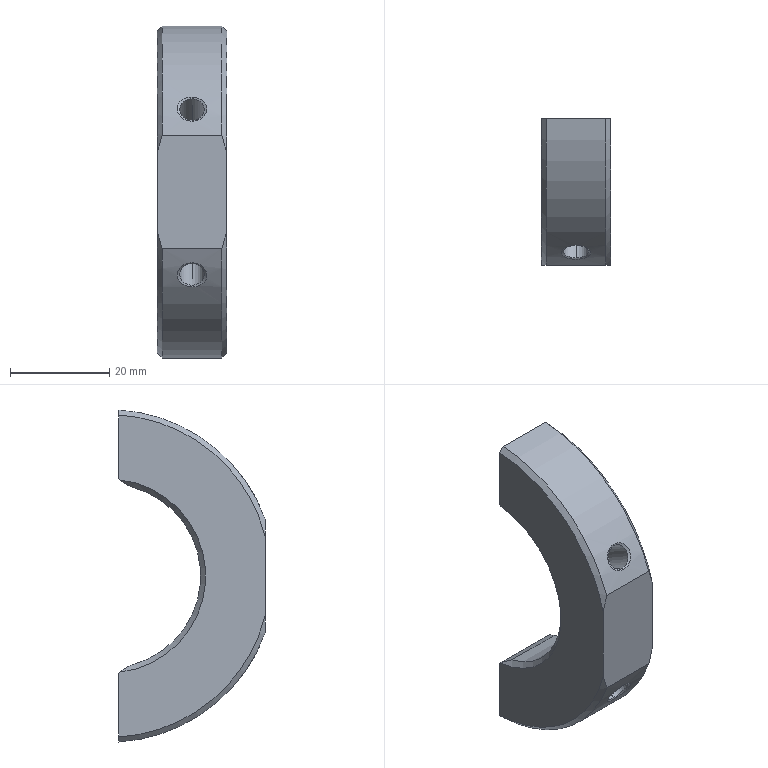Part | SolidWorks | features BaseBody 1 | 1 solid | 30 faces | box 14 x 29.5 x 66.88 mm | volume 15247 mm3 | cone 14 | plane 9 | cylinder 7 | commonest cylinder face diameters 5 x4 67 x2 37 x1
STEP:
#1=CARTESIAN_POINT('',(133.,-20.303,8.835));
#2=VERTEX_POINT('',#1);
#3=CARTESIAN_POINT('',(133.,-17.803,13.165));
#4=VERTEX_POINT('',#3);
#5=CARTESIAN_POINT('',(133.,-19.053,11.));
#6=DIRECTION('',(0.,-0.866,0.5));
#7=DIRECTION('',(0.,0.5,0.866));
#8=AXIS2_PLACEMENT_3D('',#5,#6,#7);
#9=CIRCLE('',#8,2.5);
#10=EDGE_CURVE('',#2,#4,#9,.T.);
#11=ORIENTED_EDGE('',*,*,#10,.F.);
#12=CARTESIAN_POINT('',(133.,-30.012,14.441));
#13=VERTEX_POINT('',#12);
#14=CARTESIAN_POINT('',(133.,-30.262,14.585));
#15=DIRECTION('',(0.,-0.866,0.5));
#16=VECTOR('',#15,1000.);
#17=LINE('',#14,#16);
#18=EDGE_CURVE('',#2,#13,#17,.T.);
#19=ORIENTED_EDGE('',*,*,#18,.T.);
#20=CARTESIAN_POINT('',(133.,-27.512,18.771));
#21=VERTEX_POINT('',#20);
#22=CARTESIAN_POINT('',(133.,-28.762,16.606));
#23=DIRECTION('',(0.,-0.866,0.5));
#24=DIRECTION('',(0.,0.5,0.866));
#25=AXIS2_PLACEMENT_3D('',#22,#23,#24);
#26=CIRCLE('',#25,2.5);
#27=EDGE_CURVE('',#13,#21,#26,.T.);
#28=ORIENTED_EDGE('',*,*,#27,.T.);
#29=CARTESIAN_POINT('',(133.,-27.762,18.915));
#30=DIRECTION('',(0.,-0.866,0.5));
#31=VECTOR('',#30,1000.);
#32=LINE('',#29,#31);
#33=EDGE_CURVE('',#4,#21,#32,.T.);
#34=ORIENTED_EDGE('',*,*,#33,.F.);
#35=EDGE_LOOP('',(#11,#19,#28,#34));
#36=FACE_OUTER_BOUND('',#35,.T.);
#37=CARTESIAN_POINT('',(133.,-29.012,16.75));
#38=DIRECTION('',(0.,-0.866,0.5));
#39=DIRECTION('',(0.,0.5,0.866));
#40=AXIS2_PLACEMENT_3D('',#37,#38,#39);
#41=CYLINDRICAL_SURFACE('',#40,2.5);
#42=ADVANCED_FACE('',(#36),#41,.F.);
#43=CARTESIAN_POINT('',(133.,-17.752,10.249));
#44=VERTEX_POINT('',#43);
#45=CARTESIAN_POINT('',(133.,-17.803,13.165));
#46=DIRECTION('',(0.,-0.01745,0.9998));
#47=VECTOR('',#46,1000.);
#48=LINE('',#45,#47);
#49=EDGE_CURVE('',#44,#4,#48,.T.);
#50=ORIENTED_EDGE('',*,*,#49,.F.);
#51=CARTESIAN_POINT('',(133.,-20.303,8.835));
#52=DIRECTION('',(0.,-0.8746,-0.4848));
#53=VECTOR('',#52,1000.);
#54=LINE('',#51,#53);
#55=EDGE_CURVE('',#44,#2,#54,.T.);
#56=ORIENTED_EDGE('',*,*,#55,.T.);
#57=ORIENTED_EDGE('',*,*,#10,.T.);
#58=EDGE_LOOP('',(#50,#56,#57));
#59=FACE_OUTER_BOUND('',#58,.T.);
#60=CARTESIAN_POINT('',(133.,-19.053,11.));
#61=DIRECTION('',(0.,-0.866,0.5));
#62=DIRECTION('',(0.,0.5,0.866));
#63=AXIS2_PLACEMENT_3D('',#60,#61,#62);
#64=CONICAL_SURFACE('',#63,2.5,1.03);
#65=ADVANCED_FACE('',(#59),#64,.F.);
#66=ORIENTED_EDGE('',*,*,#27,.F.);
#67=CARTESIAN_POINT('',(133.,-30.309,14.269));
#68=VERTEX_POINT('',#67);
#69=CARTESIAN_POINT('',(133.,-30.512,14.152));
#70=DIRECTION('',(0.,-0.866,-0.5));
#71=VECTOR('',#70,1000.);
#72=LINE('',#69,#71);
#73=EDGE_CURVE('',#13,#68,#72,.T.);
#74=ORIENTED_EDGE('',*,*,#73,.T.);
#75=CARTESIAN_POINT('',(133.,-27.512,19.114));
#76=VERTEX_POINT('',#75);
#77=CARTESIAN_POINT('',(133.,-27.512,19.114));
#78=CARTESIAN_POINT('',(133.19,-27.512,19.114));
#79=CARTESIAN_POINT('',(133.381,-27.522,19.1));
#80=CARTESIAN_POINT('',(133.753,-27.56,19.045));
#81=CARTESIAN_POINT('',(133.935,-27.588,19.004));
#82=CARTESIAN_POINT('',(134.292,-27.664,18.893));
#83=CARTESIAN_POINT('',(134.464,-27.711,18.824));
#84=CARTESIAN_POINT('',(134.787,-27.82,18.663));
#85=CARTESIAN_POINT('',(134.939,-27.883,18.57));
#86=CARTESIAN_POINT('',(135.224,-28.024,18.356));
#87=CARTESIAN_POINT('',(135.351,-28.1,18.238));
#88=CARTESIAN_POINT('',(135.576,-28.264,17.984));
#89=CARTESIAN_POINT('',(135.675,-28.352,17.845));
#90=CARTESIAN_POINT('',(135.835,-28.535,17.551));
#91=CARTESIAN_POINT('',(135.896,-28.628,17.399));
#92=CARTESIAN_POINT('',(135.978,-28.818,17.082));
#93=CARTESIAN_POINT('',(136.,-28.916,16.916));
#94=CARTESIAN_POINT('',(136.,-29.105,16.588));
#95=CARTESIAN_POINT('',(135.98,-29.198,16.425));
#96=CARTESIAN_POINT('',(135.897,-29.379,16.098));
#97=CARTESIAN_POINT('',(135.836,-29.465,15.939));
#98=CARTESIAN_POINT('',(135.599,-29.709,15.484));
#99=CARTESIAN_POINT('',(135.362,-29.853,15.203));
#100=CARTESIAN_POINT('',(134.94,-30.022,14.863));
#101=CARTESIAN_POINT('',(134.789,-30.072,14.763));
#102=CARTESIAN_POINT('',(134.463,-30.158,14.586));
#103=CARTESIAN_POINT('',(134.29,-30.194,14.511));
#104=CARTESIAN_POINT('',(133.76,-30.28,14.331));
#105=CARTESIAN_POINT('',(133.378,-30.309,14.269));
#106=CARTESIAN_POINT('',(133.,-30.309,14.269));
#107=B_SPLINE_CURVE_WITH_KNOTS('',3,(#77,#78,#79,#80,#81,#82,#83,#84,#85,#86,#87,#88,#89,#90,#91,#92,#93,#94,#95,#96,#97,#98,#99,#100,#101,#102,#103,#104,#105,#106),.UNSPECIFIED.,.F.,.F.,(4,2,2,2,2,2,2,2,2,2,2,2,2,2,4),(0.01163,0.01219,0.01276,0.01333,0.01389,0.01446,0.01503,0.01559,0.01616,0.01672,0.01729,0.01842,0.01899,0.01956,0.02069),.UNSPECIFIED.);
#108=EDGE_CURVE('',#76,#68,#107,.T.);
#109=ORIENTED_EDGE('',*,*,#108,.F.);
#110=CARTESIAN_POINT('',(133.,-27.512,19.348));
#111=DIRECTION('',(0.,0.,1.));
#112=VECTOR('',#111,1000.);
#113=LINE('',#110,#112);
#114=EDGE_CURVE('',#21,#76,#113,.T.);
#115=ORIENTED_EDGE('',*,*,#114,.F.);
#116=EDGE_LOOP('',(#66,#74,#109,#115));
#117=FACE_OUTER_BOUND('',#116,.T.);
#118=CARTESIAN_POINT('',(133.,-29.012,16.75));
#119=DIRECTION('',(0.,-0.866,0.5));
#120=DIRECTION('',(0.,0.5,0.866));
#121=AXIS2_PLACEMENT_3D('',#118,#119,#120);
#122=CONICAL_SURFACE('',#121,3.,1.047);
#123=ADVANCED_FACE('',(#117),#122,.F.);
#124=CARTESIAN_POINT('',(133.,-17.803,-13.165));
#125=VERTEX_POINT('',#124);
#126=CARTESIAN_POINT('',(133.,-20.303,-8.835));
#127=VERTEX_POINT('',#126);
#128=CARTESIAN_POINT('',(133.,-19.053,-11.));
#129=DIRECTION('',(0.,-0.866,-0.5));
#130=DIRECTION('',(0.,-0.5,0.866));
#131=AXIS2_PLACEMENT_3D('',#128,#129,#130);
#132=CIRCLE('',#131,2.5);
#133=EDGE_CURVE('',#125,#127,#132,.T.);
#134=ORIENTED_EDGE('',*,*,#133,.F.);
#135=CARTESIAN_POINT('',(133.,-27.512,-18.771));
#136=VERTEX_POINT('',#135);
#137=CARTESIAN_POINT('',(133.,-27.762,-18.915));
#138=DIRECTION('',(0.,-0.866,-0.5));
#139=VECTOR('',#138,1000.);
#140=LINE('',#137,#139);
#141=EDGE_CURVE('',#125,#136,#140,.T.);
#142=ORIENTED_EDGE('',*,*,#141,.T.);
#143=CARTESIAN_POINT('',(133.,-30.012,-14.441));
#144=VERTEX_POINT('',#143);
#145=CARTESIAN_POINT('',(133.,-28.762,-16.606));
#146=DIRECTION('',(0.,-0.866,-0.5));
#147=DIRECTION('',(0.,-0.5,0.866));
#148=AXIS2_PLACEMENT_3D('',#145,#146,#147);
#149=CIRCLE('',#148,2.5);
#150=EDGE_CURVE('',#136,#144,#149,.T.);
#151=ORIENTED_EDGE('',*,*,#150,.T.);
#152=CARTESIAN_POINT('',(133.,-30.262,-14.585));
#153=DIRECTION('',(0.,-0.866,-0.5));
#154=VECTOR('',#153,1000.);
#155=LINE('',#152,#154);
#156=EDGE_CURVE('',#127,#144,#155,.T.);
#157=ORIENTED_EDGE('',*,*,#156,.F.);
#158=EDGE_LOOP('',(#134,#142,#151,#157));
#159=FACE_OUTER_BOUND('',#158,.T.);
#160=CARTESIAN_POINT('',(133.,-29.012,-16.75));
#161=DIRECTION('',(0.,-0.866,-0.5));
#162=DIRECTION('',(0.,-0.5,0.866));
#163=AXIS2_PLACEMENT_3D('',#160,#161,#162);
#164=CYLINDRICAL_SURFACE('',#163,2.5);
#165=ADVANCED_FACE('',(#159),#164,.F.);
#166=CARTESIAN_POINT('',(133.,-17.752,-10.249));
#167=VERTEX_POINT('',#166);
#168=CARTESIAN_POINT('',(133.,-20.303,-8.835));
#169=DIRECTION('',(0.,-0.8746,0.4848));
#170=VECTOR('',#169,1000.);
#171=LINE('',#168,#170);
#172=EDGE_CURVE('',#167,#127,#171,.T.);
#173=ORIENTED_EDGE('',*,*,#172,.F.);
#174=CARTESIAN_POINT('',(133.,-17.803,-13.165));
#175=DIRECTION('',(0.,-0.01745,-0.9998));
#176=VECTOR('',#175,1000.);
#177=LINE('',#174,#176);
#178=EDGE_CURVE('',#167,#125,#177,.T.);
#179=ORIENTED_EDGE('',*,*,#178,.T.);
#180=ORIENTED_EDGE('',*,*,#133,.T.);
#181=EDGE_LOOP('',(#173,#179,#180));
#182=FACE_OUTER_BOUND('',#181,.T.);
#183=CARTESIAN_POINT('',(133.,-19.053,-11.));
#184=DIRECTION('',(0.,-0.866,-0.5));
#185=DIRECTION('',(0.,-0.5,0.866));
#186=AXIS2_PLACEMENT_3D('',#183,#184,#185);
#187=CONICAL_SURFACE('',#186,2.5,1.03);
#188=ADVANCED_FACE('',(#182),#187,.F.);
#189=ORIENTED_EDGE('',*,*,#150,.F.);
#190=CARTESIAN_POINT('',(133.,-27.512,-19.114));
#191=VERTEX_POINT('',#190);
#192=CARTESIAN_POINT('',(133.,-27.512,-19.348));
#193=DIRECTION('',(0.,0.,-1.));
#194=VECTOR('',#193,1000.);
#195=LINE('',#192,#194);
#196=EDGE_CURVE('',#136,#191,#195,.T.);
#197=ORIENTED_EDGE('',*,*,#196,.T.);
#198=CARTESIAN_POINT('',(133.,-30.309,-14.269));
#199=VERTEX_POINT('',#198);
#200=CARTESIAN_POINT('',(133.,-30.309,-14.269));
#201=CARTESIAN_POINT('',(133.19,-30.309,-14.269));
#202=CARTESIAN_POINT('',(133.378,-30.302,-14.284));
#203=CARTESIAN_POINT('',(133.75,-30.273,-14.345));
#204=CARTESIAN_POINT('',(133.936,-30.252,-14.391));
#205=CARTESIAN_POINT('',(134.292,-30.194,-14.511));
#206=CARTESIAN_POINT('',(134.461,-30.159,-14.585));
#207=CARTESIAN_POINT('',(134.785,-30.073,-14.761));
#208=CARTESIAN_POINT('',(134.941,-30.022,-14.864));
#209=CARTESIAN_POINT('',(135.222,-29.909,-15.09));
#210=CARTESIAN_POINT('',(135.349,-29.846,-15.214));
#211=CARTESIAN_POINT('',(135.576,-29.707,-15.485));
#212=CARTESIAN_POINT('',(135.675,-29.63,-15.631));
#213=CARTESIAN_POINT('',(135.834,-29.469,-15.934));
#214=CARTESIAN_POINT('',(135.895,-29.383,-16.091));
#215=CARTESIAN_POINT('',(135.979,-29.202,-16.417));
#216=CARTESIAN_POINT('',(136.,-29.108,-16.583));
#217=CARTESIAN_POINT('',(136.,-28.917,-16.914));
#218=CARTESIAN_POINT('',(135.979,-28.821,-17.078));
#219=CARTESIAN_POINT('',(135.897,-28.63,-17.395));
#220=CARTESIAN_POINT('',(135.835,-28.535,-17.551));
#221=CARTESIAN_POINT('',(135.676,-28.353,-17.843));
#222=CARTESIAN_POINT('',(135.579,-28.266,-17.981));
#223=CARTESIAN_POINT('',(135.352,-28.101,-18.238));
#224=CARTESIAN_POINT('',(135.222,-28.023,-18.356));
#225=CARTESIAN_POINT('',(134.942,-27.884,-18.568));
#226=CARTESIAN_POINT('',(134.787,-27.82,-18.663));
#227=CARTESIAN_POINT('',(134.461,-27.71,-18.826));
#228=CARTESIAN_POINT('',(134.291,-27.664,-18.893));
#229=CARTESIAN_POINT('',(133.936,-27.589,-19.003));
#230=CARTESIAN_POINT('',(133.751,-27.56,-19.045));
#231=CARTESIAN_POINT('',(133.378,-27.521,-19.1));
#232=CARTESIAN_POINT('',(133.19,-27.512,-19.114));
#233=CARTESIAN_POINT('',(133.,-27.512,-19.114));
#234=B_SPLINE_CURVE_WITH_KNOTS('',3,(#200,#201,#202,#203,#204,#205,#206,#207,#208,#209,#210,#211,#212,#213,#214,#215,#216,#217,#218,#219,#220,#221,#222,#223,#224,#225,#226,#227,#228,#229,#230,#231,#232,#233),.UNSPECIFIED.,.F.,.F.,(4,2,2,2,2,2,2,2,2,2,2,2,2,2,2,2,4),(0.01353,0.0141,0.01467,0.01523,0.0158,0.01637,0.01694,0.01751,0.01807,0.01864,0.01921,0.01978,0.02035,0.02091,0.02148,0.02205,0.02262),.UNSPECIFIED.);
#235=EDGE_CURVE('',#199,#191,#234,.T.);
#236=ORIENTED_EDGE('',*,*,#235,.F.);
#237=CARTESIAN_POINT('',(133.,-30.512,-14.152));
#238=DIRECTION('',(0.,-0.866,0.5));
#239=VECTOR('',#238,1000.);
#240=LINE('',#237,#239);
#241=EDGE_CURVE('',#144,#199,#240,.T.);
#242=ORIENTED_EDGE('',*,*,#241,.F.);
#243=EDGE_LOOP('',(#189,#197,#236,#242));
#244=FACE_OUTER_BOUND('',#243,.T.);
#245=CARTESIAN_POINT('',(133.,-29.012,-16.75));
#246=DIRECTION('',(0.,-0.866,-0.5));
#247=DIRECTION('',(0.,-0.5,0.866));
#248=AXIS2_PLACEMENT_3D('',#245,#246,#247);
#249=CONICAL_SURFACE('',#248,3.,1.047);
#250=ADVANCED_FACE('',(#244),#249,.F.);
#251=CARTESIAN_POINT('',(139.,-4.5,17.944));
#252=VERTEX_POINT('',#251);
#253=CARTESIAN_POINT('',(139.,-4.5,-17.944));
#254=VERTEX_POINT('',#253);
#255=CARTESIAN_POINT('',(139.,0.,0.));
#256=DIRECTION('',(1.,0.,0.));
#257=DIRECTION('',(0.,0.,1.));
#258=AXIS2_PLACEMENT_3D('',#255,#256,#257);
#259=CIRCLE('',#258,18.5);
#260=EDGE_CURVE('',#252,#254,#259,.T.);
#261=ORIENTED_EDGE('',*,*,#260,.T.);
#262=CARTESIAN_POINT('',(127.,-4.5,-17.944));
#263=VERTEX_POINT('',#262);
#264=CARTESIAN_POINT('',(140.,-4.5,-17.944));
#265=DIRECTION('',(-1.,0.,0.));
#266=VECTOR('',#265,1000.);
#267=LINE('',#264,#266);
#268=EDGE_CURVE('',#254,#263,#267,.T.);
#269=ORIENTED_EDGE('',*,*,#268,.T.);
#270=CARTESIAN_POINT('',(127.,-4.5,17.944));
#271=VERTEX_POINT('',#270);
#272=CARTESIAN_POINT('',(127.,0.,0.));
#273=DIRECTION('',(-1.,0.,0.));
#274=DIRECTION('',(0.,0.,1.));
#275=AXIS2_PLACEMENT_3D('',#272,#273,#274);
#276=CIRCLE('',#275,18.5);
#277=EDGE_CURVE('',#263,#271,#276,.T.);
#278=ORIENTED_EDGE('',*,*,#277,.T.);
#279=CARTESIAN_POINT('',(140.,-4.5,17.944));
#280=DIRECTION('',(-1.,0.,0.));
#281=VECTOR('',#280,1000.);
#282=LINE('',#279,#281);
#283=EDGE_CURVE('',#252,#271,#282,.T.);
#284=ORIENTED_EDGE('',*,*,#283,.F.);
#285=EDGE_LOOP('',(#261,#269,#278,#284));
#286=FACE_OUTER_BOUND('',#285,.T.);
#287=CARTESIAN_POINT('',(126.,0.,0.));
#288=DIRECTION('',(1.,0.,0.));
#289=DIRECTION('',(0.,0.,-1.));
#290=AXIS2_PLACEMENT_3D('',#287,#288,#289);
#291=CYLINDRICAL_SURFACE('',#290,18.5);
#292=ADVANCED_FACE('',(#286),#291,.F.);
#293=CARTESIAN_POINT('',(126.,-2.,-19.599));
#294=VERTEX_POINT('',#293);
#295=CARTESIAN_POINT('',(126.,-2.,-32.438));
#296=VERTEX_POINT('',#295);
#297=CARTESIAN_POINT('',(126.,-2.,-33.44));
#298=DIRECTION('',(0.,0.,-1.));
#299=VECTOR('',#298,1000.);
#300=LINE('',#297,#299);
#301=EDGE_CURVE('',#294,#296,#300,.T.);
#302=ORIENTED_EDGE('',*,*,#301,.F.);
#303=CARTESIAN_POINT('',(140.,-2.,-19.599));
#304=VERTEX_POINT('',#303);
#305=CARTESIAN_POINT('',(140.,-2.,-19.599));
#306=DIRECTION('',(-1.,0.,0.));
#307=VECTOR('',#306,1000.);
#308=LINE('',#305,#307);
#309=EDGE_CURVE('',#304,#294,#308,.T.);
#310=ORIENTED_EDGE('',*,*,#309,.F.);
#311=CARTESIAN_POINT('',(140.,-2.,-32.438));
#312=VERTEX_POINT('',#311);
#313=CARTESIAN_POINT('',(140.,-2.,-33.44));
#314=DIRECTION('',(0.,0.,-1.));
#315=VECTOR('',#314,1000.);
#316=LINE('',#313,#315);
#317=EDGE_CURVE('',#304,#312,#316,.T.);
#318=ORIENTED_EDGE('',*,*,#317,.T.);
#319=CARTESIAN_POINT('',(139.,-2.,-33.44));
#320=VERTEX_POINT('',#319);
#321=CARTESIAN_POINT('',(140.,-2.,-32.438));
#322=CARTESIAN_POINT('',(139.667,-2.,-32.772));
#323=CARTESIAN_POINT('',(139.333,-2.,-33.106));
#324=CARTESIAN_POINT('',(139.,-2.,-33.44));
#325=B_SPLINE_CURVE_WITH_KNOTS('',3,(#321,#322,#323,#324),.UNSPECIFIED.,.F.,.F.,(4,4),(0.,0.001416),.UNSPECIFIED.);
#326=EDGE_CURVE('',#312,#320,#325,.T.);
#327=ORIENTED_EDGE('',*,*,#326,.T.);
#328=CARTESIAN_POINT('',(127.,-2.,-33.44));
#329=VERTEX_POINT('',#328);
#330=CARTESIAN_POINT('',(126.,-2.,-33.44));
#331=DIRECTION('',(1.,0.,0.));
#332=VECTOR('',#331,1000.);
#333=LINE('',#330,#332);
#334=EDGE_CURVE('',#329,#320,#333,.T.);
#335=ORIENTED_EDGE('',*,*,#334,.F.);
#336=CARTESIAN_POINT('',(127.,-2.,-33.44));
#337=CARTESIAN_POINT('',(126.667,-2.,-33.106));
#338=CARTESIAN_POINT('',(126.333,-2.,-32.772));
#339=CARTESIAN_POINT('',(126.,-2.,-32.438));
#340=B_SPLINE_CURVE_WITH_KNOTS('',3,(#336,#337,#338,#339),.UNSPECIFIED.,.F.,.F.,(4,4),(0.,0.001416),.UNSPECIFIED.);
#341=EDGE_CURVE('',#329,#296,#340,.T.);
#342=ORIENTED_EDGE('',*,*,#341,.T.);
#343=EDGE_LOOP('',(#302,#310,#318,#327,#335,#342));
#344=FACE_OUTER_BOUND('',#343,.T.);
#345=CARTESIAN_POINT('',(126.,-2.,-33.44));
#346=DIRECTION('',(0.,-1.,0.));
#347=DIRECTION('',(1.,0.,0.));
#348=AXIS2_PLACEMENT_3D('',#345,#346,#347);
#349=PLANE('',#348);
#350=ADVANCED_FACE('',(#344),#349,.F.);
#351=ORIENTED_EDGE('',*,*,#235,.T.);
#352=CARTESIAN_POINT('',(133.,-27.512,-19.114));
#353=CARTESIAN_POINT('',(132.81,-27.512,-19.114));
#354=CARTESIAN_POINT('',(132.619,-27.522,-19.1));
#355=CARTESIAN_POINT('',(132.247,-27.56,-19.045));
#356=CARTESIAN_POINT('',(132.065,-27.588,-19.004));
#357=CARTESIAN_POINT('',(131.709,-27.664,-18.893));
#358=CARTESIAN_POINT('',(131.536,-27.711,-18.824));
#359=CARTESIAN_POINT('',(131.213,-27.82,-18.663));
#360=CARTESIAN_POINT('',(131.061,-27.883,-18.57));
#361=CARTESIAN_POINT('',(130.636,-28.094,-18.25));
#362=CARTESIAN_POINT('',(130.406,-28.26,-17.993));
#363=CARTESIAN_POINT('',(130.165,-28.535,-17.552));
#364=CARTESIAN_POINT('',(130.104,-28.628,-17.399));
#365=CARTESIAN_POINT('',(130.022,-28.818,-17.083));
#366=CARTESIAN_POINT('',(130.,-28.915,-16.917));
#367=CARTESIAN_POINT('',(130.,-29.105,-16.589));
#368=CARTESIAN_POINT('',(130.02,-29.198,-16.425));
#369=CARTESIAN_POINT('',(130.102,-29.379,-16.099));
#370=CARTESIAN_POINT('',(130.164,-29.465,-15.94));
#371=CARTESIAN_POINT('',(130.322,-29.627,-15.637));
#372=CARTESIAN_POINT('',(130.42,-29.704,-15.49));
#373=CARTESIAN_POINT('',(130.647,-29.844,-15.218));
#374=CARTESIAN_POINT('',(130.774,-29.907,-15.094));
#375=CARTESIAN_POINT('',(131.056,-30.021,-14.865));
#376=CARTESIAN_POINT('',(131.211,-30.072,-14.763));
#377=CARTESIAN_POINT('',(131.535,-30.158,-14.587));
#378=CARTESIAN_POINT('',(131.706,-30.194,-14.512));
#379=CARTESIAN_POINT('',(132.064,-30.252,-14.391));
#380=CARTESIAN_POINT('',(132.247,-30.273,-14.345));
#381=CARTESIAN_POINT('',(132.619,-30.302,-14.285));
#382=CARTESIAN_POINT('',(132.81,-30.309,-14.269));
#383=CARTESIAN_POINT('',(133.,-30.309,-14.269));
#384=B_SPLINE_CURVE_WITH_KNOTS('',3,(#352,#353,#354,#355,#356,#357,#358,#359,#360,#361,#362,#363,#364,#365,#366,#367,#368,#369,#370,#371,#372,#373,#374,#375,#376,#377,#378,#379,#380,#381,#382,#383),.UNSPECIFIED.,.F.,.F.,(4,2,2,2,2,2,2,2,2,2,2,2,2,2,2,4),(0.004439,0.005007,0.005576,0.006144,0.006712,0.007848,0.008416,0.008984,0.009552,0.01012,0.01069,0.01126,0.01182,0.01239,0.01296,0.01353),.UNSPECIFIED.);
#385=EDGE_CURVE('',#191,#199,#384,.T.);
#386=ORIENTED_EDGE('',*,*,#385,.T.);
#387=EDGE_LOOP('',(#351,#386));
#388=FACE_BOUND('',#387,.T.);
#389=ORIENTED_EDGE('',*,*,#334,.T.);
#390=CARTESIAN_POINT('',(139.,-31.5,-11.402));
#391=VERTEX_POINT('',#390);
#392=CARTESIAN_POINT('',(139.,0.,0.));
#393=DIRECTION('',(-1.,0.,0.));
#394=DIRECTION('',(0.,0.,1.));
#395=AXIS2_PLACEMENT_3D('',#392,#393,#394);
#396=CIRCLE('',#395,33.5);
#397=EDGE_CURVE('',#320,#391,#396,.T.);
#398=ORIENTED_EDGE('',*,*,#397,.T.);
#399=CARTESIAN_POINT('',(127.,-31.5,-11.402));
#400=VERTEX_POINT('',#399);
#401=CARTESIAN_POINT('',(126.,-31.5,-11.402));
#402=DIRECTION('',(1.,0.,0.));
#403=VECTOR('',#402,1000.);
#404=LINE('',#401,#403);
#405=EDGE_CURVE('',#400,#391,#404,.T.);
#406=ORIENTED_EDGE('',*,*,#405,.F.);
#407=CARTESIAN_POINT('',(127.,0.,0.));
#408=DIRECTION('',(1.,0.,0.));
#409=DIRECTION('',(0.,0.,1.));
#410=AXIS2_PLACEMENT_3D('',#407,#408,#409);
#411=CIRCLE('',#410,33.5);
#412=EDGE_CURVE('',#400,#329,#411,.T.);
#413=ORIENTED_EDGE('',*,*,#412,.T.);
#414=EDGE_LOOP('',(#389,#398,#406,#413));
#415=FACE_OUTER_BOUND('',#414,.T.);
#416=CARTESIAN_POINT('',(126.,0.,0.));
#417=DIRECTION('',(1.,0.,0.));
#418=DIRECTION('',(0.,0.,-1.));
#419=AXIS2_PLACEMENT_3D('',#416,#417,#418);
#420=CYLINDRICAL_SURFACE('',#419,33.5);
#421=ADVANCED_FACE('',(#388,#415),#420,.T.);
#422=CARTESIAN_POINT('',(140.,-31.5,-8.));
#423=VERTEX_POINT('',#422);
#424=CARTESIAN_POINT('',(140.,-31.5,8.));
#425=VERTEX_POINT('',#424);
#426=CARTESIAN_POINT('',(140.,-31.5,-11.402));
#427=DIRECTION('',(0.,0.,1.));
#428=VECTOR('',#427,1000.);
#429=LINE('',#426,#428);
#430=EDGE_CURVE('',#423,#425,#429,.T.);
#431=ORIENTED_EDGE('',*,*,#430,.T.);
#432=CARTESIAN_POINT('',(139.,-31.5,11.402));
#433=VERTEX_POINT('',#432);
#434=CARTESIAN_POINT('',(140.,-31.5,8.));
#435=CARTESIAN_POINT('',(139.717,-31.5,9.149));
#436=CARTESIAN_POINT('',(139.381,-31.5,10.282));
#437=CARTESIAN_POINT('',(139.,-31.5,11.402));
#438=B_SPLINE_CURVE_WITH_KNOTS('',3,(#434,#435,#436,#437),.UNSPECIFIED.,.F.,.F.,(4,4),(0.,0.003546),.UNSPECIFIED.);
#439=EDGE_CURVE('',#425,#433,#438,.T.);
#440=ORIENTED_EDGE('',*,*,#439,.T.);
#441=CARTESIAN_POINT('',(127.,-31.5,11.402));
#442=VERTEX_POINT('',#441);
#443=CARTESIAN_POINT('',(126.,-31.5,11.402));
#444=DIRECTION('',(1.,0.,0.));
#445=VECTOR('',#444,1000.);
#446=LINE('',#443,#445);
#447=EDGE_CURVE('',#442,#433,#446,.T.);
#448=ORIENTED_EDGE('',*,*,#447,.F.);
#449=CARTESIAN_POINT('',(126.,-31.5,8.));
#450=VERTEX_POINT('',#449);
#451=CARTESIAN_POINT('',(127.,-31.5,11.402));
#452=CARTESIAN_POINT('',(126.619,-31.5,10.282));
#453=CARTESIAN_POINT('',(126.283,-31.5,9.149));
#454=CARTESIAN_POINT('',(126.,-31.5,8.));
#455=B_SPLINE_CURVE_WITH_KNOTS('',3,(#451,#452,#453,#454),.UNSPECIFIED.,.F.,.F.,(4,4),(0.,0.003546),.UNSPECIFIED.);
#456=EDGE_CURVE('',#442,#450,#455,.T.);
#457=ORIENTED_EDGE('',*,*,#456,.T.);
#458=CARTESIAN_POINT('',(126.,-31.5,-8.));
#459=VERTEX_POINT('',#458);
#460=CARTESIAN_POINT('',(126.,-31.5,-11.402));
#461=DIRECTION('',(0.,0.,1.));
#462=VECTOR('',#461,1000.);
#463=LINE('',#460,#462);
#464=EDGE_CURVE('',#459,#450,#463,.T.);
#465=ORIENTED_EDGE('',*,*,#464,.F.);
#466=CARTESIAN_POINT('',(126.,-31.5,-8.));
#467=CARTESIAN_POINT('',(126.283,-31.5,-9.149));
#468=CARTESIAN_POINT('',(126.619,-31.5,-10.282));
#469=CARTESIAN_POINT('',(127.,-31.5,-11.402));
#470=B_SPLINE_CURVE_WITH_KNOTS('',3,(#466,#467,#468,#469),.UNSPECIFIED.,.F.,.F.,(4,4),(0.,0.003546),.UNSPECIFIED.);
#471=EDGE_CURVE('',#459,#400,#470,.T.);
#472=ORIENTED_EDGE('',*,*,#471,.T.);
#473=ORIENTED_EDGE('',*,*,#405,.T.);
#474=CARTESIAN_POINT('',(139.,-31.5,-11.402));
#475=CARTESIAN_POINT('',(139.381,-31.5,-10.282));
#476=CARTESIAN_POINT('',(139.717,-31.5,-9.149));
#477=CARTESIAN_POINT('',(140.,-31.5,-8.));
#478=B_SPLINE_CURVE_WITH_KNOTS('',3,(#474,#475,#476,#477),.UNSPECIFIED.,.F.,.F.,(4,4),(0.,0.003546),.UNSPECIFIED.);
#479=EDGE_CURVE('',#391,#423,#478,.T.);
#480=ORIENTED_EDGE('',*,*,#479,.T.);
#481=EDGE_LOOP('',(#431,#440,#448,#457,#465,#472,#473,#480));
#482=FACE_OUTER_BOUND('',#481,.T.);
#483=CARTESIAN_POINT('',(126.,-31.5,-11.402));
#484=DIRECTION('',(0.,1.,0.));
#485=DIRECTION('',(-1.,0.,0.));
#486=AXIS2_PLACEMENT_3D('',#483,#484,#485);
#487=PLANE('',#486);
#488=ADVANCED_FACE('',(#482),#487,.F.);
#489=ORIENTED_EDGE('',*,*,#108,.T.);
#490=CARTESIAN_POINT('',(133.,-30.309,14.269));
#491=CARTESIAN_POINT('',(132.811,-30.309,14.269));
#492=CARTESIAN_POINT('',(132.621,-30.302,14.284));
#493=CARTESIAN_POINT('',(132.246,-30.273,14.346));
#494=CARTESIAN_POINT('',(132.063,-30.252,14.391));
#495=CARTESIAN_POINT('',(131.71,-30.194,14.511));
#496=CARTESIAN_POINT('',(131.537,-30.158,14.586));
#497=CARTESIAN_POINT('',(131.211,-30.072,14.762));
#498=CARTESIAN_POINT('',(131.06,-30.023,14.863));
#499=CARTESIAN_POINT('',(130.779,-29.91,15.089));
#500=CARTESIAN_POINT('',(130.649,-29.845,15.216));
#501=CARTESIAN_POINT('',(130.423,-29.706,15.487));
#502=CARTESIAN_POINT('',(130.326,-29.631,15.63));
#503=CARTESIAN_POINT('',(130.166,-29.469,15.934));
#504=CARTESIAN_POINT('',(130.104,-29.381,16.094));
#505=CARTESIAN_POINT('',(130.022,-29.202,16.417));
#506=CARTESIAN_POINT('',(130.,-29.11,16.581));
#507=CARTESIAN_POINT('',(130.,-28.918,16.913));
#508=CARTESIAN_POINT('',(130.02,-28.822,17.075));
#509=CARTESIAN_POINT('',(130.102,-28.632,17.392));
#510=CARTESIAN_POINT('',(130.164,-28.536,17.549));
#511=CARTESIAN_POINT('',(130.402,-28.263,17.987));
#512=CARTESIAN_POINT('',(130.635,-28.094,18.249));
#513=CARTESIAN_POINT('',(131.057,-27.884,18.567));
#514=CARTESIAN_POINT('',(131.212,-27.821,18.662));
#515=CARTESIAN_POINT('',(131.537,-27.711,18.825));
#516=CARTESIAN_POINT('',(131.708,-27.664,18.893));
#517=CARTESIAN_POINT('',(132.063,-27.589,19.003));
#518=CARTESIAN_POINT('',(132.249,-27.56,19.045));
#519=CARTESIAN_POINT('',(132.621,-27.521,19.1));
#520=CARTESIAN_POINT('',(132.81,-27.512,19.114));
#521=CARTESIAN_POINT('',(133.,-27.512,19.114));
#522=B_SPLINE_CURVE_WITH_KNOTS('',3,(#490,#491,#492,#493,#494,#495,#496,#497,#498,#499,#500,#501,#502,#503,#504,#505,#506,#507,#508,#509,#510,#511,#512,#513,#514,#515,#516,#517,#518,#519,#520,#521),.UNSPECIFIED.,.F.,.F.,(4,2,2,2,2,2,2,2,2,2,2,2,2,2,2,4),(0.002561,0.003128,0.003694,0.004261,0.004828,0.005394,0.005961,0.006527,0.007094,0.007661,0.008227,0.009361,0.009927,0.01049,0.01106,0.01163),.UNSPECIFIED.);
#523=EDGE_CURVE('',#68,#76,#522,.T.);
#524=ORIENTED_EDGE('',*,*,#523,.T.);
#525=EDGE_LOOP('',(#489,#524));
#526=FACE_BOUND('',#525,.T.);
#527=ORIENTED_EDGE('',*,*,#447,.T.);
#528=CARTESIAN_POINT('',(139.,-2.,33.44));
#529=VERTEX_POINT('',#528);
#530=CARTESIAN_POINT('',(139.,0.,0.));
#531=DIRECTION('',(-1.,0.,0.));
#532=DIRECTION('',(0.,0.,1.));
#533=AXIS2_PLACEMENT_3D('',#530,#531,#532);
#534=CIRCLE('',#533,33.5);
#535=EDGE_CURVE('',#433,#529,#534,.T.);
#536=ORIENTED_EDGE('',*,*,#535,.T.);
#537=CARTESIAN_POINT('',(127.,-2.,33.44));
#538=VERTEX_POINT('',#537);
#539=CARTESIAN_POINT('',(126.,-2.,33.44));
#540=DIRECTION('',(1.,0.,0.));
#541=VECTOR('',#540,1000.);
#542=LINE('',#539,#541);
#543=EDGE_CURVE('',#538,#529,#542,.T.);
#544=ORIENTED_EDGE('',*,*,#543,.F.);
#545=CARTESIAN_POINT('',(127.,0.,0.));
#546=DIRECTION('',(1.,0.,0.));
#547=DIRECTION('',(0.,0.,1.));
#548=AXIS2_PLACEMENT_3D('',#545,#546,#547);
#549=CIRCLE('',#548,33.5);
#550=EDGE_CURVE('',#538,#442,#549,.T.);
#551=ORIENTED_EDGE('',*,*,#550,.T.);
#552=EDGE_LOOP('',(#527,#536,#544,#551));
#553=FACE_OUTER_BOUND('',#552,.T.);
#554=CARTESIAN_POINT('',(126.,0.,0.));
#555=DIRECTION('',(1.,0.,0.));
#556=DIRECTION('',(0.,0.,-1.));
#557=AXIS2_PLACEMENT_3D('',#554,#555,#556);
#558=CYLINDRICAL_SURFACE('',#557,33.5);
#559=ADVANCED_FACE('',(#526,#553),#558,.T.);
#560=CARTESIAN_POINT('',(140.,-2.,32.438));
#561=VERTEX_POINT('',#560);
#562=CARTESIAN_POINT('',(140.,-2.,19.599));
#563=VERTEX_POINT('',#562);
#564=CARTESIAN_POINT('',(140.,-2.,18.392));
#565=DIRECTION('',(0.,0.,-1.));
#566=VECTOR('',#565,1000.);
#567=LINE('',#564,#566);
#568=EDGE_CURVE('',#561,#563,#567,.T.);
#569=ORIENTED_EDGE('',*,*,#568,.T.);
#570=CARTESIAN_POINT('',(126.,-2.,19.599));
#571=VERTEX_POINT('',#570);
#572=CARTESIAN_POINT('',(140.,-2.,19.599));
#573=DIRECTION('',(-1.,0.,0.));
#574=VECTOR('',#573,1000.);
#575=LINE('',#572,#574);
#576=EDGE_CURVE('',#563,#571,#575,.T.);
#577=ORIENTED_EDGE('',*,*,#576,.T.);
#578=CARTESIAN_POINT('',(126.,-2.,32.438));
#579=VERTEX_POINT('',#578);
#580=CARTESIAN_POINT('',(126.,-2.,18.392));
#581=DIRECTION('',(0.,0.,-1.));
#582=VECTOR('',#581,1000.);
#583=LINE('',#580,#582);
#584=EDGE_CURVE('',#579,#571,#583,.T.);
#585=ORIENTED_EDGE('',*,*,#584,.F.);
#586=CARTESIAN_POINT('',(126.,-2.,32.438));
#587=CARTESIAN_POINT('',(126.333,-2.,32.772));
#588=CARTESIAN_POINT('',(126.667,-2.,33.106));
#589=CARTESIAN_POINT('',(127.,-2.,33.44));
#590=B_SPLINE_CURVE_WITH_KNOTS('',3,(#586,#587,#588,#589),.UNSPECIFIED.,.F.,.F.,(4,4),(0.,0.001416),.UNSPECIFIED.);
#591=EDGE_CURVE('',#579,#538,#590,.T.);
#592=ORIENTED_EDGE('',*,*,#591,.T.);
#593=ORIENTED_EDGE('',*,*,#543,.T.);
#594=CARTESIAN_POINT('',(139.,-2.,33.44));
#595=CARTESIAN_POINT('',(139.333,-2.,33.106));
#596=CARTESIAN_POINT('',(139.667,-2.,32.772));
#597=CARTESIAN_POINT('',(140.,-2.,32.438));
#598=B_SPLINE_CURVE_WITH_KNOTS('',3,(#594,#595,#596,#597),.UNSPECIFIED.,.F.,.F.,(4,4),(0.,0.001416),.UNSPECIFIED.);
#599=EDGE_CURVE('',#529,#561,#598,.T.);
#600=ORIENTED_EDGE('',*,*,#599,.T.);
#601=EDGE_LOOP('',(#569,#577,#585,#592,#593,#600));
#602=FACE_OUTER_BOUND('',#601,.T.);
#603=CARTESIAN_POINT('',(126.,-2.,18.392));
#604=DIRECTION('',(0.,-1.,0.));
#605=DIRECTION('',(1.,0.,0.));
#606=AXIS2_PLACEMENT_3D('',#603,#604,#605);
#607=PLANE('',#606);
#608=ADVANCED_FACE('',(#602),#607,.F.);
#609=CARTESIAN_POINT('',(126.,-2.227,-19.372));
#610=VERTEX_POINT('',#609);
#611=CARTESIAN_POINT('',(126.,-2.5,-19.099));
#612=DIRECTION('',(0.,-0.7071,0.7071));
#613=VECTOR('',#612,1000.);
#614=LINE('',#611,#613);
#615=EDGE_CURVE('',#294,#610,#614,.T.);
#616=ORIENTED_EDGE('',*,*,#615,.F.);
#617=ORIENTED_EDGE('',*,*,#301,.T.);
#618=CARTESIAN_POINT('',(126.,0.,0.));
#619=DIRECTION('',(-1.,0.,0.));
#620=DIRECTION('',(0.,0.,1.));
#621=AXIS2_PLACEMENT_3D('',#618,#619,#620);
#622=CIRCLE('',#621,32.5);
#623=EDGE_CURVE('',#296,#459,#622,.T.);
#624=ORIENTED_EDGE('',*,*,#623,.T.);
#625=ORIENTED_EDGE('',*,*,#464,.T.);
#626=CARTESIAN_POINT('',(126.,0.,0.));
#627=DIRECTION('',(-1.,0.,0.));
#628=DIRECTION('',(0.,0.,1.));
#629=AXIS2_PLACEMENT_3D('',#626,#627,#628);
#630=CIRCLE('',#629,32.5);
#631=EDGE_CURVE('',#450,#579,#630,.T.);
#632=ORIENTED_EDGE('',*,*,#631,.T.);
#633=ORIENTED_EDGE('',*,*,#584,.T.);
#634=CARTESIAN_POINT('',(126.,-2.227,19.372));
#635=VERTEX_POINT('',#634);
#636=CARTESIAN_POINT('',(126.,-2.5,19.099));
#637=DIRECTION('',(0.,0.7071,0.7071));
#638=VECTOR('',#637,1000.);
#639=LINE('',#636,#638);
#640=EDGE_CURVE('',#635,#571,#639,.T.);
#641=ORIENTED_EDGE('',*,*,#640,.F.);
#642=CARTESIAN_POINT('',(126.,0.,0.));
#643=DIRECTION('',(1.,0.,0.));
#644=DIRECTION('',(0.,0.,1.));
#645=AXIS2_PLACEMENT_3D('',#642,#643,#644);
#646=CIRCLE('',#645,19.5);
#647=EDGE_CURVE('',#635,#610,#646,.T.);
#648=ORIENTED_EDGE('',*,*,#647,.T.);
#649=EDGE_LOOP('',(#616,#617,#624,#625,#632,#633,#641,#648));
#650=FACE_OUTER_BOUND('',#649,.T.);
#651=CARTESIAN_POINT('',(126.,0.,0.));
#652=DIRECTION('',(-1.,0.,0.));
#653=DIRECTION('',(0.,0.,1.));
#654=AXIS2_PLACEMENT_3D('',#651,#652,#653);
#655=PLANE('',#654);
#656=ADVANCED_FACE('',(#650),#655,.T.);
#657=ORIENTED_EDGE('',*,*,#317,.F.);
#658=CARTESIAN_POINT('',(140.,-2.227,-19.372));
#659=VERTEX_POINT('',#658);
#660=CARTESIAN_POINT('',(140.,-2.5,-19.099));
#661=DIRECTION('',(0.,-0.7071,0.7071));
#662=VECTOR('',#661,1000.);
#663=LINE('',#660,#662);
#664=EDGE_CURVE('',#304,#659,#663,.T.);
#665=ORIENTED_EDGE('',*,*,#664,.T.);
#666=CARTESIAN_POINT('',(140.,-2.227,19.372));
#667=VERTEX_POINT('',#666);
#668=CARTESIAN_POINT('',(140.,0.,0.));
#669=DIRECTION('',(-1.,0.,0.));
#670=DIRECTION('',(0.,0.,1.));
#671=AXIS2_PLACEMENT_3D('',#668,#669,#670);
#672=CIRCLE('',#671,19.5);
#673=EDGE_CURVE('',#659,#667,#672,.T.);
#674=ORIENTED_EDGE('',*,*,#673,.T.);
#675=CARTESIAN_POINT('',(140.,-2.5,19.099));
#676=DIRECTION('',(0.,0.7071,0.7071));
#677=VECTOR('',#676,1000.);
#678=LINE('',#675,#677);
#679=EDGE_CURVE('',#667,#563,#678,.T.);
#680=ORIENTED_EDGE('',*,*,#679,.T.);
#681=ORIENTED_EDGE('',*,*,#568,.F.);
#682=CARTESIAN_POINT('',(140.,0.,0.));
#683=DIRECTION('',(1.,0.,0.));
#684=DIRECTION('',(0.,0.,1.));
#685=AXIS2_PLACEMENT_3D('',#682,#683,#684);
#686=CIRCLE('',#685,32.5);
#687=EDGE_CURVE('',#561,#425,#686,.T.);
#688=ORIENTED_EDGE('',*,*,#687,.T.);
#689=ORIENTED_EDGE('',*,*,#430,.F.);
#690=CARTESIAN_POINT('',(140.,0.,0.));
#691=DIRECTION('',(1.,0.,0.));
#692=DIRECTION('',(0.,0.,1.));
#693=AXIS2_PLACEMENT_3D('',#690,#691,#692);
#694=CIRCLE('',#693,32.5);
#695=EDGE_CURVE('',#423,#312,#694,.T.);
#696=ORIENTED_EDGE('',*,*,#695,.T.);
#697=EDGE_LOOP('',(#657,#665,#674,#680,#681,#688,#689,#696));
#698=FACE_OUTER_BOUND('',#697,.T.);
#699=CARTESIAN_POINT('',(140.,0.,0.));
#700=DIRECTION('',(-1.,0.,0.));
#701=DIRECTION('',(0.,0.,1.));
#702=AXIS2_PLACEMENT_3D('',#699,#700,#701);
#703=PLANE('',#702);
#704=ADVANCED_FACE('',(#698),#703,.F.);
#705=CARTESIAN_POINT('',(126.238,-2.5,-19.099));
#706=VERTEX_POINT('',#705);
#707=CARTESIAN_POINT('',(126.238,-2.5,-19.099));
#708=CARTESIAN_POINT('',(126.529,-3.156,-18.72));
#709=CARTESIAN_POINT('',(126.785,-3.822,-18.336));
#710=CARTESIAN_POINT('',(127.,-4.5,-17.944));
#711=B_SPLINE_CURVE_WITH_KNOTS('',3,(#707,#708,#709,#710),.UNSPECIFIED.,.F.,.F.,(4,4),(0.000000247,0.002432),.UNSPECIFIED.);
#712=EDGE_CURVE('',#706,#263,#711,.T.);
#713=ORIENTED_EDGE('',*,*,#712,.F.);
#714=CARTESIAN_POINT('',(126.,-2.227,-19.372));
#715=CARTESIAN_POINT('',(126.08,-2.317,-19.282));
#716=CARTESIAN_POINT('',(126.159,-2.409,-19.19));
#717=CARTESIAN_POINT('',(126.238,-2.5,-19.099));
#718=B_SPLINE_CURVE_WITH_KNOTS('',3,(#714,#715,#716,#717),.UNSPECIFIED.,.F.,.F.,(4,4),(0.000000379,0.0004544),.UNSPECIFIED.);
#719=EDGE_CURVE('',#610,#706,#718,.T.);
#720=ORIENTED_EDGE('',*,*,#719,.F.);
#721=ORIENTED_EDGE('',*,*,#647,.F.);
#722=CARTESIAN_POINT('',(126.238,-2.5,19.099));
#723=VERTEX_POINT('',#722);
#724=CARTESIAN_POINT('',(126.238,-2.5,19.099));
#725=CARTESIAN_POINT('',(126.159,-2.409,19.19));
#726=CARTESIAN_POINT('',(126.08,-2.317,19.282));
#727=CARTESIAN_POINT('',(126.,-2.227,19.372));
#728=B_SPLINE_CURVE_WITH_KNOTS('',3,(#724,#725,#726,#727),.UNSPECIFIED.,.F.,.F.,(4,4),(0.000000331,0.0004544),.UNSPECIFIED.);
#729=EDGE_CURVE('',#723,#635,#728,.T.);
#730=ORIENTED_EDGE('',*,*,#729,.F.);
#731=CARTESIAN_POINT('',(127.,-4.5,17.944));
#732=CARTESIAN_POINT('',(126.785,-3.822,18.336));
#733=CARTESIAN_POINT('',(126.529,-3.156,18.72));
#734=CARTESIAN_POINT('',(126.238,-2.5,19.099));
#735=B_SPLINE_CURVE_WITH_KNOTS('',3,(#731,#732,#733,#734),.UNSPECIFIED.,.F.,.F.,(4,4),(0.000000239,0.002432),.UNSPECIFIED.);
#736=EDGE_CURVE('',#271,#723,#735,.T.);
#737=ORIENTED_EDGE('',*,*,#736,.F.);
#738=ORIENTED_EDGE('',*,*,#277,.F.);
#739=EDGE_LOOP('',(#713,#720,#721,#730,#737,#738));
#740=FACE_OUTER_BOUND('',#739,.T.);
#741=CARTESIAN_POINT('',(126.,0.,0.));
#742=DIRECTION('',(-1.,0.,0.));
#743=DIRECTION('',(0.,0.,1.));
#744=AXIS2_PLACEMENT_3D('',#741,#742,#743);
#745=CONICAL_SURFACE('',#744,19.5,0.7854);
#746=ADVANCED_FACE('',(#740),#745,.F.);
#747=CARTESIAN_POINT('',(139.762,-2.5,-19.099));
#748=VERTEX_POINT('',#747);
#749=CARTESIAN_POINT('',(139.,-4.5,-17.944));
#750=CARTESIAN_POINT('',(139.215,-3.822,-18.336));
#751=CARTESIAN_POINT('',(139.471,-3.156,-18.72));
#752=CARTESIAN_POINT('',(139.762,-2.5,-19.099));
#753=B_SPLINE_CURVE_WITH_KNOTS('',3,(#749,#750,#751,#752),.UNSPECIFIED.,.F.,.F.,(4,4),(0.000000239,0.002432),.UNSPECIFIED.);
#754=EDGE_CURVE('',#254,#748,#753,.T.);
#755=ORIENTED_EDGE('',*,*,#754,.F.);
#756=ORIENTED_EDGE('',*,*,#260,.F.);
#757=CARTESIAN_POINT('',(139.762,-2.5,19.099));
#758=VERTEX_POINT('',#757);
#759=CARTESIAN_POINT('',(139.762,-2.5,19.099));
#760=CARTESIAN_POINT('',(139.471,-3.156,18.72));
#761=CARTESIAN_POINT('',(139.215,-3.822,18.336));
#762=CARTESIAN_POINT('',(139.,-4.5,17.944));
#763=B_SPLINE_CURVE_WITH_KNOTS('',3,(#759,#760,#761,#762),.UNSPECIFIED.,.F.,.F.,(4,4),(0.000000247,0.002432),.UNSPECIFIED.);
#764=EDGE_CURVE('',#758,#252,#763,.T.);
#765=ORIENTED_EDGE('',*,*,#764,.F.);
#766=CARTESIAN_POINT('',(140.,-2.227,19.372));
#767=CARTESIAN_POINT('',(139.92,-2.317,19.282));
#768=CARTESIAN_POINT('',(139.841,-2.409,19.19));
#769=CARTESIAN_POINT('',(139.762,-2.5,19.099));
#770=B_SPLINE_CURVE_WITH_KNOTS('',3,(#766,#767,#768,#769),.UNSPECIFIED.,.F.,.F.,(4,4),(0.000000379,0.0004544),.UNSPECIFIED.);
#771=EDGE_CURVE('',#667,#758,#770,.T.);
#772=ORIENTED_EDGE('',*,*,#771,.F.);
#773=ORIENTED_EDGE('',*,*,#673,.F.);
#774=CARTESIAN_POINT('',(139.762,-2.5,-19.099));
#775=CARTESIAN_POINT('',(139.841,-2.409,-19.19));
#776=CARTESIAN_POINT('',(139.92,-2.317,-19.282));
#777=CARTESIAN_POINT('',(140.,-2.227,-19.372));
#778=B_SPLINE_CURVE_WITH_KNOTS('',3,(#774,#775,#776,#777),.UNSPECIFIED.,.F.,.F.,(4,4),(0.000000331,0.0004544),.UNSPECIFIED.);
#779=EDGE_CURVE('',#748,#659,#778,.T.);
#780=ORIENTED_EDGE('',*,*,#779,.F.);
#781=EDGE_LOOP('',(#755,#756,#765,#772,#773,#780));
#782=FACE_OUTER_BOUND('',#781,.T.);
#783=CARTESIAN_POINT('',(139.,0.,0.));
#784=DIRECTION('',(1.,0.,0.));
#785=DIRECTION('',(0.,0.,-1.));
#786=AXIS2_PLACEMENT_3D('',#783,#784,#785);
#787=CONICAL_SURFACE('',#786,18.5,0.7854);
#788=ADVANCED_FACE('',(#782),#787,.F.);
#789=ORIENTED_EDGE('',*,*,#439,.F.);
#790=ORIENTED_EDGE('',*,*,#687,.F.);
#791=ORIENTED_EDGE('',*,*,#599,.F.);
#792=ORIENTED_EDGE('',*,*,#535,.F.);
#793=EDGE_LOOP('',(#789,#790,#791,#792));
#794=FACE_OUTER_BOUND('',#793,.T.);
#795=CARTESIAN_POINT('',(139.,0.,0.));
#796=DIRECTION('',(-1.,0.,0.));
#797=DIRECTION('',(0.,0.,1.));
#798=AXIS2_PLACEMENT_3D('',#795,#796,#797);
#799=CONICAL_SURFACE('',#798,33.5,0.7854);
#800=ADVANCED_FACE('',(#794),#799,.T.);
#801=ORIENTED_EDGE('',*,*,#456,.F.);
#802=ORIENTED_EDGE('',*,*,#550,.F.);
#803=ORIENTED_EDGE('',*,*,#591,.F.);
#804=ORIENTED_EDGE('',*,*,#631,.F.);
#805=EDGE_LOOP('',(#801,#802,#803,#804));
#806=FACE_OUTER_BOUND('',#805,.T.);
#807=CARTESIAN_POINT('',(126.,0.,0.));
#808=DIRECTION('',(1.,0.,0.));
#809=DIRECTION('',(0.,0.,-1.));
#810=AXIS2_PLACEMENT_3D('',#807,#808,#809);
#811=CONICAL_SURFACE('',#810,32.5,0.7854);
#812=ADVANCED_FACE('',(#806),#811,.T.);
#813=ORIENTED_EDGE('',*,*,#326,.F.);
#814=ORIENTED_EDGE('',*,*,#695,.F.);
#815=ORIENTED_EDGE('',*,*,#479,.F.);
#816=ORIENTED_EDGE('',*,*,#397,.F.);
#817=EDGE_LOOP('',(#813,#814,#815,#816));
#818=FACE_OUTER_BOUND('',#817,.T.);
#819=CARTESIAN_POINT('',(139.,0.,0.));
#820=DIRECTION('',(-1.,0.,0.));
#821=DIRECTION('',(0.,0.,1.));
#822=AXIS2_PLACEMENT_3D('',#819,#820,#821);
#823=CONICAL_SURFACE('',#822,33.5,0.7854);
#824=ADVANCED_FACE('',(#818),#823,.T.);
#825=ORIENTED_EDGE('',*,*,#341,.F.);
#826=ORIENTED_EDGE('',*,*,#412,.F.);
#827=ORIENTED_EDGE('',*,*,#471,.F.);
#828=ORIENTED_EDGE('',*,*,#623,.F.);
#829=EDGE_LOOP('',(#825,#826,#827,#828));
#830=FACE_OUTER_BOUND('',#829,.T.);
#831=CARTESIAN_POINT('',(126.,0.,0.));
#832=DIRECTION('',(1.,0.,0.));
#833=DIRECTION('',(0.,0.,-1.));
#834=AXIS2_PLACEMENT_3D('',#831,#832,#833);
#835=CONICAL_SURFACE('',#834,32.5,0.7854);
#836=ADVANCED_FACE('',(#830),#835,.T.);
#837=ORIENTED_EDGE('',*,*,#736,.T.);
#838=CARTESIAN_POINT('',(140.,-2.5,19.099));
#839=DIRECTION('',(-1.,0.,0.));
#840=VECTOR('',#839,1000.);
#841=LINE('',#838,#840);
#842=EDGE_CURVE('',#758,#723,#841,.T.);
#843=ORIENTED_EDGE('',*,*,#842,.F.);
#844=ORIENTED_EDGE('',*,*,#764,.T.);
#845=ORIENTED_EDGE('',*,*,#283,.T.);
#846=EDGE_LOOP('',(#837,#843,#844,#845));
#847=FACE_OUTER_BOUND('',#846,.T.);
#848=CARTESIAN_POINT('',(140.,-4.5,17.944));
#849=DIRECTION('',(0.,-0.5,0.866));
#850=DIRECTION('',(0.,0.866,0.5));
#851=AXIS2_PLACEMENT_3D('',#848,#849,#850);
#852=PLANE('',#851);
#853=ADVANCED_FACE('',(#847),#852,.F.);
#854=ORIENTED_EDGE('',*,*,#729,.T.);
#855=ORIENTED_EDGE('',*,*,#640,.T.);
#856=ORIENTED_EDGE('',*,*,#576,.F.);
#857=ORIENTED_EDGE('',*,*,#679,.F.);
#858=ORIENTED_EDGE('',*,*,#771,.T.);
#859=ORIENTED_EDGE('',*,*,#842,.T.);
#860=EDGE_LOOP('',(#854,#855,#856,#857,#858,#859));
#861=FACE_OUTER_BOUND('',#860,.T.);
#862=CARTESIAN_POINT('',(140.,-2.5,19.099));
#863=DIRECTION('',(0.,-0.7071,0.7071));
#864=DIRECTION('',(0.,0.7071,0.7071));
#865=AXIS2_PLACEMENT_3D('',#862,#863,#864);
#866=PLANE('',#865);
#867=ADVANCED_FACE('',(#861),#866,.F.);
#868=ORIENTED_EDGE('',*,*,#712,.T.);
#869=ORIENTED_EDGE('',*,*,#268,.F.);
#870=ORIENTED_EDGE('',*,*,#754,.T.);
#871=CARTESIAN_POINT('',(140.,-2.5,-19.099));
#872=DIRECTION('',(-1.,0.,0.));
#873=VECTOR('',#872,1000.);
#874=LINE('',#871,#873);
#875=EDGE_CURVE('',#748,#706,#874,.T.);
#876=ORIENTED_EDGE('',*,*,#875,.T.);
#877=EDGE_LOOP('',(#868,#869,#870,#876));
#878=FACE_OUTER_BOUND('',#877,.T.);
#879=CARTESIAN_POINT('',(140.,-4.5,-17.944));
#880=DIRECTION('',(0.,-0.5,-0.866));
#881=DIRECTION('',(0.,-0.866,0.5));
#882=AXIS2_PLACEMENT_3D('',#879,#880,#881);
#883=PLANE('',#882);
#884=ADVANCED_FACE('',(#878),#883,.F.);
#885=ORIENTED_EDGE('',*,*,#719,.T.);
#886=ORIENTED_EDGE('',*,*,#875,.F.);
#887=ORIENTED_EDGE('',*,*,#779,.T.);
#888=ORIENTED_EDGE('',*,*,#664,.F.);
#889=ORIENTED_EDGE('',*,*,#309,.T.);
#890=ORIENTED_EDGE('',*,*,#615,.T.);
#891=EDGE_LOOP('',(#885,#886,#887,#888,#889,#890));
#892=FACE_OUTER_BOUND('',#891,.T.);
#893=CARTESIAN_POINT('',(140.,-2.5,-19.099));
#894=DIRECTION('',(0.,-0.7071,-0.7071));
#895=DIRECTION('',(0.,-0.7071,0.7071));
#896=AXIS2_PLACEMENT_3D('',#893,#894,#895);
#897=PLANE('',#896);
#898=ADVANCED_FACE('',(#892),#897,.F.);
#899=ORIENTED_EDGE('',*,*,#196,.F.);
#900=CARTESIAN_POINT('',(133.,-28.762,-16.606));
#901=DIRECTION('',(0.,-0.866,-0.5));
#902=DIRECTION('',(0.,-0.5,0.866));
#903=AXIS2_PLACEMENT_3D('',#900,#901,#902);
#904=CIRCLE('',#903,2.5);
#905=EDGE_CURVE('',#144,#136,#904,.T.);
#906=ORIENTED_EDGE('',*,*,#905,.F.);
#907=ORIENTED_EDGE('',*,*,#241,.T.);
#908=ORIENTED_EDGE('',*,*,#385,.F.);
#909=EDGE_LOOP('',(#899,#906,#907,#908));
#910=FACE_OUTER_BOUND('',#909,.T.);
#911=CARTESIAN_POINT('',(133.,-29.012,-16.75));
#912=DIRECTION('',(0.,-0.866,-0.5));
#913=DIRECTION('',(0.,-0.5,0.866));
#914=AXIS2_PLACEMENT_3D('',#911,#912,#913);
#915=CONICAL_SURFACE('',#914,3.,1.047);
#916=ADVANCED_FACE('',(#910),#915,.F.);
#917=ORIENTED_EDGE('',*,*,#178,.F.);
#918=ORIENTED_EDGE('',*,*,#172,.T.);
#919=CARTESIAN_POINT('',(133.,-19.053,-11.));
#920=DIRECTION('',(0.,-0.866,-0.5));
#921=DIRECTION('',(0.,-0.5,0.866));
#922=AXIS2_PLACEMENT_3D('',#919,#920,#921);
#923=CIRCLE('',#922,2.5);
#924=EDGE_CURVE('',#127,#125,#923,.T.);
#925=ORIENTED_EDGE('',*,*,#924,.T.);
#926=EDGE_LOOP('',(#917,#918,#925));
#927=FACE_OUTER_BOUND('',#926,.T.);
#928=CARTESIAN_POINT('',(133.,-19.053,-11.));
#929=DIRECTION('',(0.,-0.866,-0.5));
#930=DIRECTION('',(0.,-0.5,0.866));
#931=AXIS2_PLACEMENT_3D('',#928,#929,#930);
#932=CONICAL_SURFACE('',#931,2.5,1.03);
#933=ADVANCED_FACE('',(#927),#932,.F.);
#934=ORIENTED_EDGE('',*,*,#141,.F.);
#935=ORIENTED_EDGE('',*,*,#924,.F.);
#936=ORIENTED_EDGE('',*,*,#156,.T.);
#937=ORIENTED_EDGE('',*,*,#905,.T.);
#938=EDGE_LOOP('',(#934,#935,#936,#937));
#939=FACE_OUTER_BOUND('',#938,.T.);
#940=CARTESIAN_POINT('',(133.,-29.012,-16.75));
#941=DIRECTION('',(0.,-0.866,-0.5));
#942=DIRECTION('',(0.,-0.5,0.866));
#943=AXIS2_PLACEMENT_3D('',#940,#941,#942);
#944=CYLINDRICAL_SURFACE('',#943,2.5);
#945=ADVANCED_FACE('',(#939),#944,.F.);
#946=ORIENTED_EDGE('',*,*,#73,.F.);
#947=CARTESIAN_POINT('',(133.,-28.762,16.606));
#948=DIRECTION('',(0.,-0.866,0.5));
#949=DIRECTION('',(0.,0.5,0.866));
#950=AXIS2_PLACEMENT_3D('',#947,#948,#949);
#951=CIRCLE('',#950,2.5);
#952=EDGE_CURVE('',#21,#13,#951,.T.);
#953=ORIENTED_EDGE('',*,*,#952,.F.);
#954=ORIENTED_EDGE('',*,*,#114,.T.);
#955=ORIENTED_EDGE('',*,*,#523,.F.);
#956=EDGE_LOOP('',(#946,#953,#954,#955));
#957=FACE_OUTER_BOUND('',#956,.T.);
#958=CARTESIAN_POINT('',(133.,-29.012,16.75));
#959=DIRECTION('',(0.,-0.866,0.5));
#960=DIRECTION('',(0.,0.5,0.866));
#961=AXIS2_PLACEMENT_3D('',#958,#959,#960);
#962=CONICAL_SURFACE('',#961,3.,1.047);
#963=ADVANCED_FACE('',(#957),#962,.F.);
#964=ORIENTED_EDGE('',*,*,#55,.F.);
#965=ORIENTED_EDGE('',*,*,#49,.T.);
#966=CARTESIAN_POINT('',(133.,-19.053,11.));
#967=DIRECTION('',(0.,-0.866,0.5));
#968=DIRECTION('',(0.,0.5,0.866));
#969=AXIS2_PLACEMENT_3D('',#966,#967,#968);
#970=CIRCLE('',#969,2.5);
#971=EDGE_CURVE('',#4,#2,#970,.T.);
#972=ORIENTED_EDGE('',*,*,#971,.T.);
#973=EDGE_LOOP('',(#964,#965,#972));
#974=FACE_OUTER_BOUND('',#973,.T.);
#975=CARTESIAN_POINT('',(133.,-19.053,11.));
#976=DIRECTION('',(0.,-0.866,0.5));
#977=DIRECTION('',(0.,0.5,0.866));
#978=AXIS2_PLACEMENT_3D('',#975,#976,#977);
#979=CONICAL_SURFACE('',#978,2.5,1.03);
#980=ADVANCED_FACE('',(#974),#979,.F.);
#981=ORIENTED_EDGE('',*,*,#18,.F.);
#982=ORIENTED_EDGE('',*,*,#971,.F.);
#983=ORIENTED_EDGE('',*,*,#33,.T.);
#984=ORIENTED_EDGE('',*,*,#952,.T.);
#985=EDGE_LOOP('',(#981,#982,#983,#984));
#986=FACE_OUTER_BOUND('',#985,.T.);
#987=CARTESIAN_POINT('',(133.,-29.012,16.75));
#988=DIRECTION('',(0.,-0.866,0.5));
#989=DIRECTION('',(0.,0.5,0.866));
#990=AXIS2_PLACEMENT_3D('',#987,#988,#989);
#991=CYLINDRICAL_SURFACE('',#990,2.5);
#992=ADVANCED_FACE('',(#986),#991,.F.);
#993=CLOSED_SHELL('',(#42,#65,#123,#165,#188,#250,#292,#350,#421,#488,#559,#608,#656,#704,#746,#788,#800,#812,#824,#836,#853,#867,#884,#898,#916,#933,#945,#963,#980,#992));
#994=MANIFOLD_SOLID_BREP('',#993);
#995=CARTESIAN_POINT('',(0.,0.,0.));
#996=DIRECTION('',(0.,0.,1.));
#997=DIRECTION('',(1.,0.,0.));
#998=AXIS2_PLACEMENT_3D('',#995,#996,#997);
#999=(LENGTH_UNIT()NAMED_UNIT(*)SI_UNIT(.MILLI.,.METRE.));
#1000=UNCERTAINTY_MEASURE_WITH_UNIT(LENGTH_MEASURE(0.00001),#999,'','');
#1001=(NAMED_UNIT(*)PLANE_ANGLE_UNIT()SI_UNIT($,.RADIAN.));
#1002=(NAMED_UNIT(*)SI_UNIT($,.STERADIAN.)SOLID_ANGLE_UNIT());
#1003=(GEOMETRIC_REPRESENTATION_CONTEXT(3)GLOBAL_UNCERTAINTY_ASSIGNED_CONTEXT((#1000))GLOBAL_UNIT_ASSIGNED_CONTEXT((#999,#1001,#1002))REPRESENTATION_CONTEXT('',''));
#1004=ADVANCED_BREP_SHAPE_REPRESENTATION('',(#994,#998),#1003);